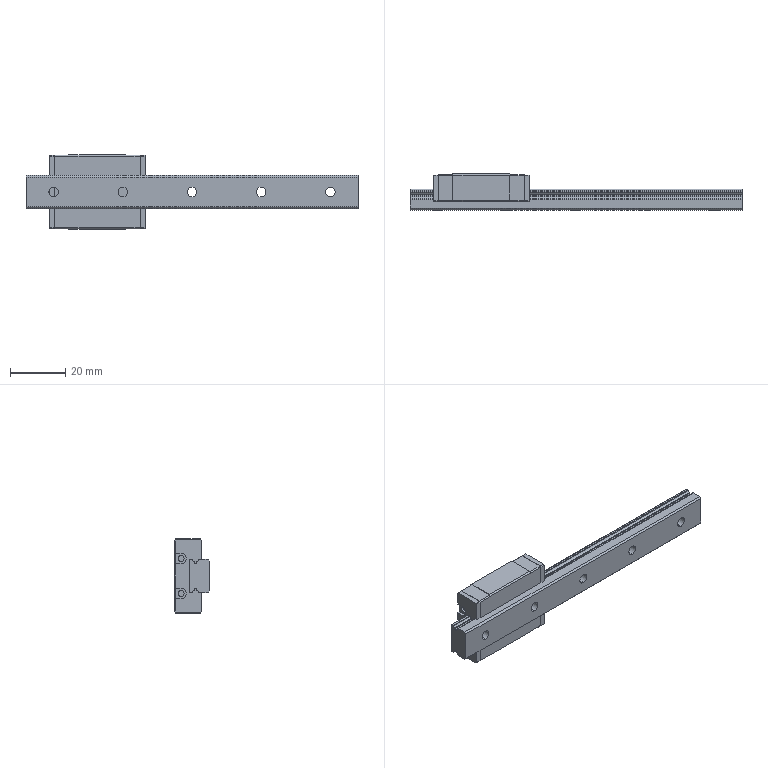Part | NX | features BREP 4 | 4 solids | 1540 faces | box 120 x 13 x 27 mm | volume 16651 mm3 | plane 1415 | cylinder 109 | cone 16 | commonest cylinder face diameters 0.4 x32 2.571 x16 0.8 x12 3.5 x10 6 x10 0.6 x8